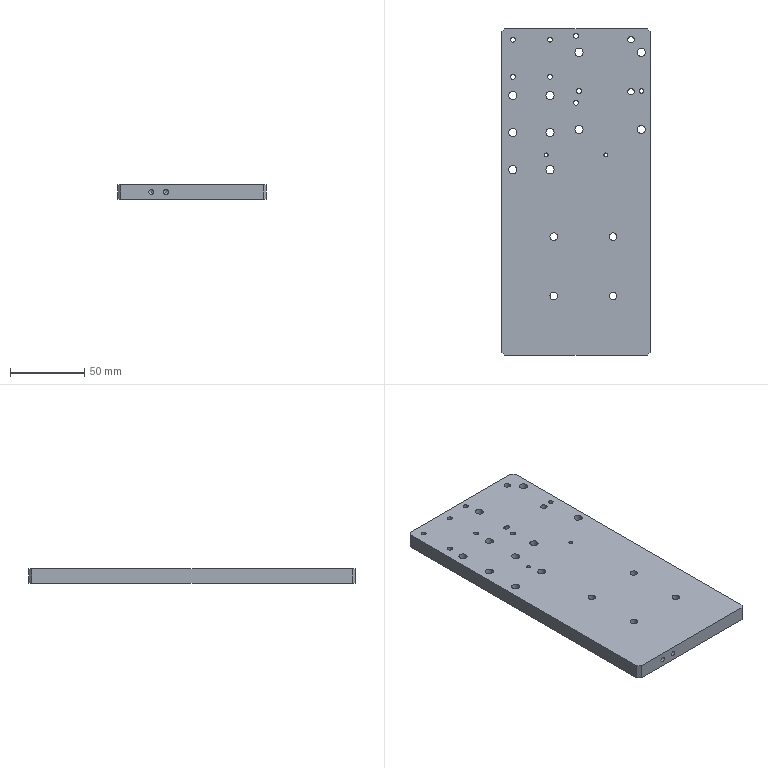Part | 1 solid | 67 faces | box 100 x 220 x 10 mm | volume 212133 mm3 | cylinder 41 | plane 22 | cone 4 | commonest cylinder face diameters 5.5 x10 10 x10 3.3 x8 5 x4 3 x3 2.5 x2